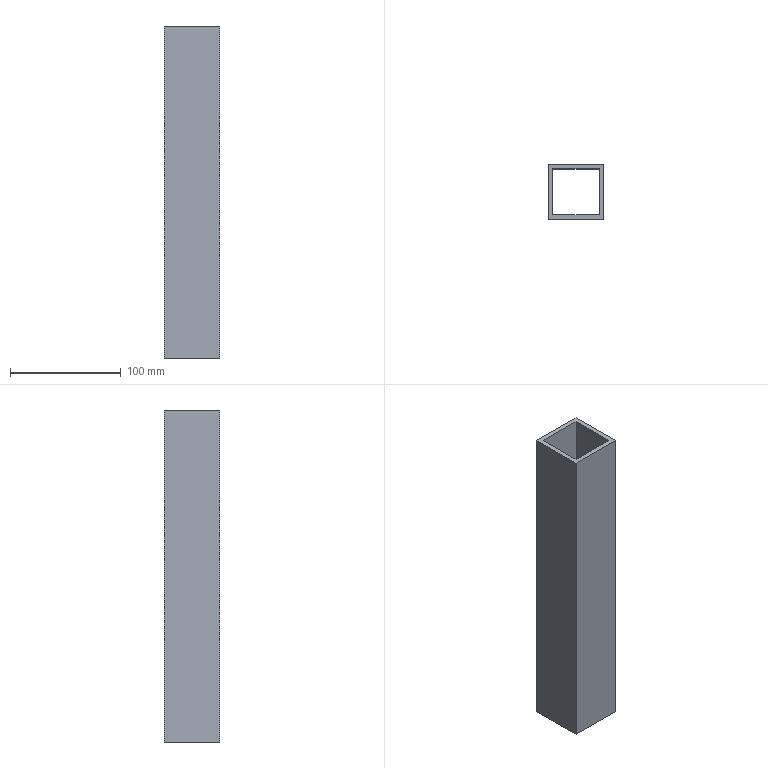Part | STEP file | PN_0083 straight stop bar | 1 solid | 10 faces | box 50 x 50 x 300 mm | volume 220800 mm3 | plane 10
STEP:
#1=CARTESIAN_POINT('',(0.,0.,0.));
#2=DIRECTION('',(0.,0.,1.));
#3=DIRECTION('',(1.,0.,0.));
#4=AXIS2_PLACEMENT_3D('',#1,#2,#3);
#5=CARTESIAN_POINT('',(-25.,25.,300.));
#6=VERTEX_POINT('',#5);
#7=CARTESIAN_POINT('',(-25.,-25.,300.));
#8=VERTEX_POINT('',#7);
#9=CARTESIAN_POINT('',(-25.,-25.,300.));
#10=DIRECTION('',(0.,-1.,0.));
#11=VECTOR('',#10,1.);
#12=LINE('',#9,#11);
#13=CARTESIAN_POINT('',(0.,0.,300.));
#14=DIRECTION('',(0.,0.,1.));
#15=DIRECTION('',(1.,0.,0.));
#16=AXIS2_PLACEMENT_3D('',#13,#14,#15);
#17=PLANE('',#16);
#18=CARTESIAN_POINT('',(-25.,-25.));
#19=DIRECTION('',(0.,-1.));
#20=VECTOR('',#19,1.);
#21=LINE('',#18,#20);
#22=(GEOMETRIC_REPRESENTATION_CONTEXT(2)PARAMETRIC_REPRESENTATION_CONTEXT()REPRESENTATION_CONTEXT('',''));
#23=DEFINITIONAL_REPRESENTATION('',(#21),#22);
#24=PCURVE('',#17,#23);
#25=CARTESIAN_POINT('',(-25.,-25.,300.));
#26=DIRECTION('',(1.,0.,0.));
#27=DIRECTION('',(0.,0.,-1.));
#28=AXIS2_PLACEMENT_3D('',#25,#26,#27);
#29=PLANE('',#28);
#30=CARTESIAN_POINT('',(0.,0.));
#31=DIRECTION('',(0.,-1.));
#32=VECTOR('',#31,1.);
#33=LINE('',#30,#32);
#34=(GEOMETRIC_REPRESENTATION_CONTEXT(2)PARAMETRIC_REPRESENTATION_CONTEXT()REPRESENTATION_CONTEXT('',''));
#35=DEFINITIONAL_REPRESENTATION('',(#33),#34);
#36=PCURVE('',#29,#35);
#37=SURFACE_CURVE('',#12,(#24,#36),.PCURVE_S1.);
#38=EDGE_CURVE('',#6,#8,#37,.T.);
#39=ORIENTED_EDGE('',*,*,#38,.T.);
#40=CARTESIAN_POINT('',(25.,-25.,300.));
#41=VERTEX_POINT('',#40);
#42=CARTESIAN_POINT('',(25.,-25.,300.));
#43=DIRECTION('',(1.,0.,0.));
#44=VECTOR('',#43,1.);
#45=LINE('',#42,#44);
#46=CARTESIAN_POINT('',(25.,-25.));
#47=DIRECTION('',(1.,0.));
#48=VECTOR('',#47,1.);
#49=LINE('',#46,#48);
#50=(GEOMETRIC_REPRESENTATION_CONTEXT(2)PARAMETRIC_REPRESENTATION_CONTEXT()REPRESENTATION_CONTEXT('',''));
#51=DEFINITIONAL_REPRESENTATION('',(#49),#50);
#52=PCURVE('',#17,#51);
#53=CARTESIAN_POINT('',(25.,-25.,300.));
#54=DIRECTION('',(0.,1.,0.));
#55=DIRECTION('',(-1.,0.,0.));
#56=AXIS2_PLACEMENT_3D('',#53,#54,#55);
#57=PLANE('',#56);
#58=CARTESIAN_POINT('',(0.,0.));
#59=DIRECTION('',(-1.,0.));
#60=VECTOR('',#59,1.);
#61=LINE('',#58,#60);
#62=(GEOMETRIC_REPRESENTATION_CONTEXT(2)PARAMETRIC_REPRESENTATION_CONTEXT()REPRESENTATION_CONTEXT('',''));
#63=DEFINITIONAL_REPRESENTATION('',(#61),#62);
#64=PCURVE('',#57,#63);
#65=SURFACE_CURVE('',#45,(#52,#64),.PCURVE_S1.);
#66=EDGE_CURVE('',#8,#41,#65,.T.);
#67=ORIENTED_EDGE('',*,*,#66,.T.);
#68=CARTESIAN_POINT('',(25.,25.,300.));
#69=VERTEX_POINT('',#68);
#70=CARTESIAN_POINT('',(25.,-25.,300.));
#71=DIRECTION('',(0.,1.,0.));
#72=VECTOR('',#71,1.);
#73=LINE('',#70,#72);
#74=CARTESIAN_POINT('',(25.,-25.));
#75=DIRECTION('',(0.,1.));
#76=VECTOR('',#75,1.);
#77=LINE('',#74,#76);
#78=(GEOMETRIC_REPRESENTATION_CONTEXT(2)PARAMETRIC_REPRESENTATION_CONTEXT()REPRESENTATION_CONTEXT('',''));
#79=DEFINITIONAL_REPRESENTATION('',(#77),#78);
#80=PCURVE('',#17,#79);
#81=CARTESIAN_POINT('',(25.,-25.,300.));
#82=DIRECTION('',(-1.,0.,0.));
#83=DIRECTION('',(0.,0.,1.));
#84=AXIS2_PLACEMENT_3D('',#81,#82,#83);
#85=PLANE('',#84);
#86=CARTESIAN_POINT('',(0.,0.));
#87=DIRECTION('',(0.,1.));
#88=VECTOR('',#87,1.);
#89=LINE('',#86,#88);
#90=(GEOMETRIC_REPRESENTATION_CONTEXT(2)PARAMETRIC_REPRESENTATION_CONTEXT()REPRESENTATION_CONTEXT('',''));
#91=DEFINITIONAL_REPRESENTATION('',(#89),#90);
#92=PCURVE('',#85,#91);
#93=SURFACE_CURVE('',#73,(#80,#92),.PCURVE_S1.);
#94=EDGE_CURVE('',#41,#69,#93,.T.);
#95=ORIENTED_EDGE('',*,*,#94,.T.);
#96=CARTESIAN_POINT('',(25.,25.,300.));
#97=DIRECTION('',(-1.,0.,0.));
#98=VECTOR('',#97,1.);
#99=LINE('',#96,#98);
#100=CARTESIAN_POINT('',(25.,25.));
#101=DIRECTION('',(-1.,0.));
#102=VECTOR('',#101,1.);
#103=LINE('',#100,#102);
#104=(GEOMETRIC_REPRESENTATION_CONTEXT(2)PARAMETRIC_REPRESENTATION_CONTEXT()REPRESENTATION_CONTEXT('',''));
#105=DEFINITIONAL_REPRESENTATION('',(#103),#104);
#106=PCURVE('',#17,#105);
#107=CARTESIAN_POINT('',(25.,25.,300.));
#108=DIRECTION('',(0.,-1.,0.));
#109=DIRECTION('',(1.,0.,0.));
#110=AXIS2_PLACEMENT_3D('',#107,#108,#109);
#111=PLANE('',#110);
#112=CARTESIAN_POINT('',(0.,0.));
#113=DIRECTION('',(-1.,0.));
#114=VECTOR('',#113,1.);
#115=LINE('',#112,#114);
#116=(GEOMETRIC_REPRESENTATION_CONTEXT(2)PARAMETRIC_REPRESENTATION_CONTEXT()REPRESENTATION_CONTEXT('',''));
#117=DEFINITIONAL_REPRESENTATION('',(#115),#116);
#118=PCURVE('',#111,#117);
#119=SURFACE_CURVE('',#99,(#106,#118),.PCURVE_S1.);
#120=EDGE_CURVE('',#69,#6,#119,.T.);
#121=ORIENTED_EDGE('',*,*,#120,.T.);
#122=EDGE_LOOP('',(#39,#67,#95,#121));
#123=FACE_BOUND('',#122,.T.);
#124=CARTESIAN_POINT('',(-21.,-21.,300.));
#125=VERTEX_POINT('',#124);
#126=CARTESIAN_POINT('',(21.,-21.,300.));
#127=VERTEX_POINT('',#126);
#128=CARTESIAN_POINT('',(21.,-21.,300.));
#129=DIRECTION('',(1.,0.,0.));
#130=VECTOR('',#129,1.);
#131=LINE('',#128,#130);
#132=CARTESIAN_POINT('',(21.,-21.));
#133=DIRECTION('',(1.,0.));
#134=VECTOR('',#133,1.);
#135=LINE('',#132,#134);
#136=(GEOMETRIC_REPRESENTATION_CONTEXT(2)PARAMETRIC_REPRESENTATION_CONTEXT()REPRESENTATION_CONTEXT('',''));
#137=DEFINITIONAL_REPRESENTATION('',(#135),#136);
#138=PCURVE('',#17,#137);
#139=CARTESIAN_POINT('',(21.,-21.,300.));
#140=DIRECTION('',(0.,1.,0.));
#141=DIRECTION('',(0.,0.,1.));
#142=AXIS2_PLACEMENT_3D('',#139,#140,#141);
#143=PLANE('',#142);
#144=CARTESIAN_POINT('',(0.,0.));
#145=DIRECTION('',(0.,1.));
#146=VECTOR('',#145,1.);
#147=LINE('',#144,#146);
#148=(GEOMETRIC_REPRESENTATION_CONTEXT(2)PARAMETRIC_REPRESENTATION_CONTEXT()REPRESENTATION_CONTEXT('',''));
#149=DEFINITIONAL_REPRESENTATION('',(#147),#148);
#150=PCURVE('',#143,#149);
#151=SURFACE_CURVE('',#131,(#138,#150),.PCURVE_S1.);
#152=EDGE_CURVE('',#125,#127,#151,.T.);
#153=ORIENTED_EDGE('',*,*,#152,.F.);
#154=CARTESIAN_POINT('',(-21.,21.,300.));
#155=VERTEX_POINT('',#154);
#156=CARTESIAN_POINT('',(-21.,-21.,300.));
#157=DIRECTION('',(0.,-1.,0.));
#158=VECTOR('',#157,1.);
#159=LINE('',#156,#158);
#160=CARTESIAN_POINT('',(-21.,-21.));
#161=DIRECTION('',(0.,-1.));
#162=VECTOR('',#161,1.);
#163=LINE('',#160,#162);
#164=(GEOMETRIC_REPRESENTATION_CONTEXT(2)PARAMETRIC_REPRESENTATION_CONTEXT()REPRESENTATION_CONTEXT('',''));
#165=DEFINITIONAL_REPRESENTATION('',(#163),#164);
#166=PCURVE('',#17,#165);
#167=CARTESIAN_POINT('',(-21.,-21.,300.));
#168=DIRECTION('',(1.,0.,0.));
#169=DIRECTION('',(0.,0.,-1.));
#170=AXIS2_PLACEMENT_3D('',#167,#168,#169);
#171=PLANE('',#170);
#172=CARTESIAN_POINT('',(0.,0.));
#173=DIRECTION('',(0.,-1.));
#174=VECTOR('',#173,1.);
#175=LINE('',#172,#174);
#176=(GEOMETRIC_REPRESENTATION_CONTEXT(2)PARAMETRIC_REPRESENTATION_CONTEXT()REPRESENTATION_CONTEXT('',''));
#177=DEFINITIONAL_REPRESENTATION('',(#175),#176);
#178=PCURVE('',#171,#177);
#179=SURFACE_CURVE('',#159,(#166,#178),.PCURVE_S1.);
#180=EDGE_CURVE('',#155,#125,#179,.T.);
#181=ORIENTED_EDGE('',*,*,#180,.F.);
#182=CARTESIAN_POINT('',(21.,21.,300.));
#183=VERTEX_POINT('',#182);
#184=CARTESIAN_POINT('',(21.,21.,300.));
#185=DIRECTION('',(-1.,0.,0.));
#186=VECTOR('',#185,1.);
#187=LINE('',#184,#186);
#188=CARTESIAN_POINT('',(21.,21.));
#189=DIRECTION('',(-1.,0.));
#190=VECTOR('',#189,1.);
#191=LINE('',#188,#190);
#192=(GEOMETRIC_REPRESENTATION_CONTEXT(2)PARAMETRIC_REPRESENTATION_CONTEXT()REPRESENTATION_CONTEXT('',''));
#193=DEFINITIONAL_REPRESENTATION('',(#191),#192);
#194=PCURVE('',#17,#193);
#195=CARTESIAN_POINT('',(21.,21.,300.));
#196=DIRECTION('',(0.,-1.,0.));
#197=DIRECTION('',(0.,0.,-1.));
#198=AXIS2_PLACEMENT_3D('',#195,#196,#197);
#199=PLANE('',#198);
#200=CARTESIAN_POINT('',(0.,0.));
#201=DIRECTION('',(0.,-1.));
#202=VECTOR('',#201,1.);
#203=LINE('',#200,#202);
#204=(GEOMETRIC_REPRESENTATION_CONTEXT(2)PARAMETRIC_REPRESENTATION_CONTEXT()REPRESENTATION_CONTEXT('',''));
#205=DEFINITIONAL_REPRESENTATION('',(#203),#204);
#206=PCURVE('',#199,#205);
#207=SURFACE_CURVE('',#187,(#194,#206),.PCURVE_S1.);
#208=EDGE_CURVE('',#183,#155,#207,.T.);
#209=ORIENTED_EDGE('',*,*,#208,.F.);
#210=CARTESIAN_POINT('',(21.,-21.,300.));
#211=DIRECTION('',(0.,1.,0.));
#212=VECTOR('',#211,1.);
#213=LINE('',#210,#212);
#214=CARTESIAN_POINT('',(21.,-21.));
#215=DIRECTION('',(0.,1.));
#216=VECTOR('',#215,1.);
#217=LINE('',#214,#216);
#218=(GEOMETRIC_REPRESENTATION_CONTEXT(2)PARAMETRIC_REPRESENTATION_CONTEXT()REPRESENTATION_CONTEXT('',''));
#219=DEFINITIONAL_REPRESENTATION('',(#217),#218);
#220=PCURVE('',#17,#219);
#221=CARTESIAN_POINT('',(21.,-21.,300.));
#222=DIRECTION('',(-1.,0.,0.));
#223=DIRECTION('',(0.,0.,1.));
#224=AXIS2_PLACEMENT_3D('',#221,#222,#223);
#225=PLANE('',#224);
#226=CARTESIAN_POINT('',(0.,0.));
#227=DIRECTION('',(0.,1.));
#228=VECTOR('',#227,1.);
#229=LINE('',#226,#228);
#230=(GEOMETRIC_REPRESENTATION_CONTEXT(2)PARAMETRIC_REPRESENTATION_CONTEXT()REPRESENTATION_CONTEXT('',''));
#231=DEFINITIONAL_REPRESENTATION('',(#229),#230);
#232=PCURVE('',#225,#231);
#233=SURFACE_CURVE('',#213,(#220,#232),.PCURVE_S1.);
#234=EDGE_CURVE('',#127,#183,#233,.T.);
#235=ORIENTED_EDGE('',*,*,#234,.F.);
#236=EDGE_LOOP('',(#153,#181,#209,#235));
#237=FACE_BOUND('',#236,.T.);
#238=ADVANCED_FACE('',(#123,#237),#17,.T.);
#239=CARTESIAN_POINT('',(-25.,25.,0.));
#240=VERTEX_POINT('',#239);
#241=CARTESIAN_POINT('',(-25.,-25.,0.));
#242=VERTEX_POINT('',#241);
#243=CARTESIAN_POINT('',(-25.,-25.,0.));
#244=DIRECTION('',(0.,-1.,0.));
#245=VECTOR('',#244,1.);
#246=LINE('',#243,#245);
#247=CARTESIAN_POINT('',(0.,0.,0.));
#248=DIRECTION('',(0.,0.,1.));
#249=DIRECTION('',(1.,0.,0.));
#250=AXIS2_PLACEMENT_3D('',#247,#248,#249);
#251=PLANE('',#250);
#252=CARTESIAN_POINT('',(-25.,-25.));
#253=DIRECTION('',(0.,-1.));
#254=VECTOR('',#253,1.);
#255=LINE('',#252,#254);
#256=(GEOMETRIC_REPRESENTATION_CONTEXT(2)PARAMETRIC_REPRESENTATION_CONTEXT()REPRESENTATION_CONTEXT('',''));
#257=DEFINITIONAL_REPRESENTATION('',(#255),#256);
#258=PCURVE('',#251,#257);
#259=CARTESIAN_POINT('',(300.,0.));
#260=DIRECTION('',(0.,-1.));
#261=VECTOR('',#260,1.);
#262=LINE('',#259,#261);
#263=(GEOMETRIC_REPRESENTATION_CONTEXT(2)PARAMETRIC_REPRESENTATION_CONTEXT()REPRESENTATION_CONTEXT('',''));
#264=DEFINITIONAL_REPRESENTATION('',(#262),#263);
#265=PCURVE('',#29,#264);
#266=SURFACE_CURVE('',#246,(#258,#265),.PCURVE_S1.);
#267=EDGE_CURVE('',#240,#242,#266,.T.);
#268=ORIENTED_EDGE('',*,*,#267,.F.);
#269=CARTESIAN_POINT('',(25.,25.,0.));
#270=VERTEX_POINT('',#269);
#271=CARTESIAN_POINT('',(25.,25.,0.));
#272=DIRECTION('',(-1.,0.,0.));
#273=VECTOR('',#272,1.);
#274=LINE('',#271,#273);
#275=CARTESIAN_POINT('',(25.,25.));
#276=DIRECTION('',(-1.,0.));
#277=VECTOR('',#276,1.);
#278=LINE('',#275,#277);
#279=(GEOMETRIC_REPRESENTATION_CONTEXT(2)PARAMETRIC_REPRESENTATION_CONTEXT()REPRESENTATION_CONTEXT('',''));
#280=DEFINITIONAL_REPRESENTATION('',(#278),#279);
#281=PCURVE('',#251,#280);
#282=CARTESIAN_POINT('',(0.,-300.));
#283=DIRECTION('',(-1.,0.));
#284=VECTOR('',#283,1.);
#285=LINE('',#282,#284);
#286=(GEOMETRIC_REPRESENTATION_CONTEXT(2)PARAMETRIC_REPRESENTATION_CONTEXT()REPRESENTATION_CONTEXT('',''));
#287=DEFINITIONAL_REPRESENTATION('',(#285),#286);
#288=PCURVE('',#111,#287);
#289=SURFACE_CURVE('',#274,(#281,#288),.PCURVE_S1.);
#290=EDGE_CURVE('',#270,#240,#289,.T.);
#291=ORIENTED_EDGE('',*,*,#290,.F.);
#292=CARTESIAN_POINT('',(25.,-25.,0.));
#293=VERTEX_POINT('',#292);
#294=CARTESIAN_POINT('',(25.,-25.,0.));
#295=DIRECTION('',(0.,1.,0.));
#296=VECTOR('',#295,1.);
#297=LINE('',#294,#296);
#298=CARTESIAN_POINT('',(25.,-25.));
#299=DIRECTION('',(0.,1.));
#300=VECTOR('',#299,1.);
#301=LINE('',#298,#300);
#302=(GEOMETRIC_REPRESENTATION_CONTEXT(2)PARAMETRIC_REPRESENTATION_CONTEXT()REPRESENTATION_CONTEXT('',''));
#303=DEFINITIONAL_REPRESENTATION('',(#301),#302);
#304=PCURVE('',#251,#303);
#305=CARTESIAN_POINT('',(-300.,0.));
#306=DIRECTION('',(0.,1.));
#307=VECTOR('',#306,1.);
#308=LINE('',#305,#307);
#309=(GEOMETRIC_REPRESENTATION_CONTEXT(2)PARAMETRIC_REPRESENTATION_CONTEXT()REPRESENTATION_CONTEXT('',''));
#310=DEFINITIONAL_REPRESENTATION('',(#308),#309);
#311=PCURVE('',#85,#310);
#312=SURFACE_CURVE('',#297,(#304,#311),.PCURVE_S1.);
#313=EDGE_CURVE('',#293,#270,#312,.T.);
#314=ORIENTED_EDGE('',*,*,#313,.F.);
#315=CARTESIAN_POINT('',(25.,-25.,0.));
#316=DIRECTION('',(1.,0.,0.));
#317=VECTOR('',#316,1.);
#318=LINE('',#315,#317);
#319=CARTESIAN_POINT('',(25.,-25.));
#320=DIRECTION('',(1.,0.));
#321=VECTOR('',#320,1.);
#322=LINE('',#319,#321);
#323=(GEOMETRIC_REPRESENTATION_CONTEXT(2)PARAMETRIC_REPRESENTATION_CONTEXT()REPRESENTATION_CONTEXT('',''));
#324=DEFINITIONAL_REPRESENTATION('',(#322),#323);
#325=PCURVE('',#251,#324);
#326=CARTESIAN_POINT('',(0.,-300.));
#327=DIRECTION('',(-1.,0.));
#328=VECTOR('',#327,1.);
#329=LINE('',#326,#328);
#330=(GEOMETRIC_REPRESENTATION_CONTEXT(2)PARAMETRIC_REPRESENTATION_CONTEXT()REPRESENTATION_CONTEXT('',''));
#331=DEFINITIONAL_REPRESENTATION('',(#329),#330);
#332=PCURVE('',#57,#331);
#333=SURFACE_CURVE('',#318,(#325,#332),.PCURVE_S1.);
#334=EDGE_CURVE('',#242,#293,#333,.T.);
#335=ORIENTED_EDGE('',*,*,#334,.F.);
#336=EDGE_LOOP('',(#268,#291,#314,#335));
#337=FACE_BOUND('',#336,.T.);
#338=CARTESIAN_POINT('',(-21.,21.,0.));
#339=VERTEX_POINT('',#338);
#340=CARTESIAN_POINT('',(-21.,-21.,0.));
#341=VERTEX_POINT('',#340);
#342=CARTESIAN_POINT('',(-21.,-21.,0.));
#343=DIRECTION('',(0.,-1.,0.));
#344=VECTOR('',#343,1.);
#345=LINE('',#342,#344);
#346=CARTESIAN_POINT('',(-21.,-21.));
#347=DIRECTION('',(0.,-1.));
#348=VECTOR('',#347,1.);
#349=LINE('',#346,#348);
#350=(GEOMETRIC_REPRESENTATION_CONTEXT(2)PARAMETRIC_REPRESENTATION_CONTEXT()REPRESENTATION_CONTEXT('',''));
#351=DEFINITIONAL_REPRESENTATION('',(#349),#350);
#352=PCURVE('',#251,#351);
#353=CARTESIAN_POINT('',(300.,0.));
#354=DIRECTION('',(0.,-1.));
#355=VECTOR('',#354,1.);
#356=LINE('',#353,#355);
#357=(GEOMETRIC_REPRESENTATION_CONTEXT(2)PARAMETRIC_REPRESENTATION_CONTEXT()REPRESENTATION_CONTEXT('',''));
#358=DEFINITIONAL_REPRESENTATION('',(#356),#357);
#359=PCURVE('',#171,#358);
#360=SURFACE_CURVE('',#345,(#352,#359),.PCURVE_S1.);
#361=EDGE_CURVE('',#339,#341,#360,.T.);
#362=ORIENTED_EDGE('',*,*,#361,.T.);
#363=CARTESIAN_POINT('',(21.,-21.,0.));
#364=VERTEX_POINT('',#363);
#365=CARTESIAN_POINT('',(21.,-21.,0.));
#366=DIRECTION('',(1.,0.,0.));
#367=VECTOR('',#366,1.);
#368=LINE('',#365,#367);
#369=CARTESIAN_POINT('',(21.,-21.));
#370=DIRECTION('',(1.,0.));
#371=VECTOR('',#370,1.);
#372=LINE('',#369,#371);
#373=(GEOMETRIC_REPRESENTATION_CONTEXT(2)PARAMETRIC_REPRESENTATION_CONTEXT()REPRESENTATION_CONTEXT('',''));
#374=DEFINITIONAL_REPRESENTATION('',(#372),#373);
#375=PCURVE('',#251,#374);
#376=CARTESIAN_POINT('',(-300.,0.));
#377=DIRECTION('',(0.,1.));
#378=VECTOR('',#377,1.);
#379=LINE('',#376,#378);
#380=(GEOMETRIC_REPRESENTATION_CONTEXT(2)PARAMETRIC_REPRESENTATION_CONTEXT()REPRESENTATION_CONTEXT('',''));
#381=DEFINITIONAL_REPRESENTATION('',(#379),#380);
#382=PCURVE('',#143,#381);
#383=SURFACE_CURVE('',#368,(#375,#382),.PCURVE_S1.);
#384=EDGE_CURVE('',#341,#364,#383,.T.);
#385=ORIENTED_EDGE('',*,*,#384,.T.);
#386=CARTESIAN_POINT('',(21.,21.,0.));
#387=VERTEX_POINT('',#386);
#388=CARTESIAN_POINT('',(21.,-21.,0.));
#389=DIRECTION('',(0.,1.,0.));
#390=VECTOR('',#389,1.);
#391=LINE('',#388,#390);
#392=CARTESIAN_POINT('',(21.,-21.));
#393=DIRECTION('',(0.,1.));
#394=VECTOR('',#393,1.);
#395=LINE('',#392,#394);
#396=(GEOMETRIC_REPRESENTATION_CONTEXT(2)PARAMETRIC_REPRESENTATION_CONTEXT()REPRESENTATION_CONTEXT('',''));
#397=DEFINITIONAL_REPRESENTATION('',(#395),#396);
#398=PCURVE('',#251,#397);
#399=CARTESIAN_POINT('',(-300.,0.));
#400=DIRECTION('',(0.,1.));
#401=VECTOR('',#400,1.);
#402=LINE('',#399,#401);
#403=(GEOMETRIC_REPRESENTATION_CONTEXT(2)PARAMETRIC_REPRESENTATION_CONTEXT()REPRESENTATION_CONTEXT('',''));
#404=DEFINITIONAL_REPRESENTATION('',(#402),#403);
#405=PCURVE('',#225,#404);
#406=SURFACE_CURVE('',#391,(#398,#405),.PCURVE_S1.);
#407=EDGE_CURVE('',#364,#387,#406,.T.);
#408=ORIENTED_EDGE('',*,*,#407,.T.);
#409=CARTESIAN_POINT('',(21.,21.,0.));
#410=DIRECTION('',(-1.,0.,0.));
#411=VECTOR('',#410,1.);
#412=LINE('',#409,#411);
#413=CARTESIAN_POINT('',(21.,21.));
#414=DIRECTION('',(-1.,0.));
#415=VECTOR('',#414,1.);
#416=LINE('',#413,#415);
#417=(GEOMETRIC_REPRESENTATION_CONTEXT(2)PARAMETRIC_REPRESENTATION_CONTEXT()REPRESENTATION_CONTEXT('',''));
#418=DEFINITIONAL_REPRESENTATION('',(#416),#417);
#419=PCURVE('',#251,#418);
#420=CARTESIAN_POINT('',(300.,0.));
#421=DIRECTION('',(0.,-1.));
#422=VECTOR('',#421,1.);
#423=LINE('',#420,#422);
#424=(GEOMETRIC_REPRESENTATION_CONTEXT(2)PARAMETRIC_REPRESENTATION_CONTEXT()REPRESENTATION_CONTEXT('',''));
#425=DEFINITIONAL_REPRESENTATION('',(#423),#424);
#426=PCURVE('',#199,#425);
#427=SURFACE_CURVE('',#412,(#419,#426),.PCURVE_S1.);
#428=EDGE_CURVE('',#387,#339,#427,.T.);
#429=ORIENTED_EDGE('',*,*,#428,.T.);
#430=EDGE_LOOP('',(#362,#385,#408,#429));
#431=FACE_BOUND('',#430,.T.);
#432=ADVANCED_FACE('',(#337,#431),#251,.F.);
#433=ORIENTED_EDGE('',*,*,#267,.T.);
#434=CARTESIAN_POINT('',(-25.,-25.,300.));
#435=DIRECTION('',(0.,0.,-1.));
#436=VECTOR('',#435,1.);
#437=LINE('',#434,#436);
#438=CARTESIAN_POINT('',(0.,0.));
#439=DIRECTION('',(1.,0.));
#440=VECTOR('',#439,1.);
#441=LINE('',#438,#440);
#442=(GEOMETRIC_REPRESENTATION_CONTEXT(2)PARAMETRIC_REPRESENTATION_CONTEXT()REPRESENTATION_CONTEXT('',''));
#443=DEFINITIONAL_REPRESENTATION('',(#441),#442);
#444=PCURVE('',#29,#443);
#445=CARTESIAN_POINT('',(50.,0.));
#446=DIRECTION('',(0.,-1.));
#447=VECTOR('',#446,1.);
#448=LINE('',#445,#447);
#449=(GEOMETRIC_REPRESENTATION_CONTEXT(2)PARAMETRIC_REPRESENTATION_CONTEXT()REPRESENTATION_CONTEXT('',''));
#450=DEFINITIONAL_REPRESENTATION('',(#448),#449);
#451=PCURVE('',#57,#450);
#452=SURFACE_CURVE('',#437,(#444,#451),.PCURVE_S1.);
#453=EDGE_CURVE('',#8,#242,#452,.T.);
#454=ORIENTED_EDGE('',*,*,#453,.F.);
#455=ORIENTED_EDGE('',*,*,#38,.F.);
#456=CARTESIAN_POINT('',(-25.,25.,300.));
#457=DIRECTION('',(0.,0.,-1.));
#458=VECTOR('',#457,1.);
#459=LINE('',#456,#458);
#460=CARTESIAN_POINT('',(0.,50.));
#461=DIRECTION('',(1.,0.));
#462=VECTOR('',#461,1.);
#463=LINE('',#460,#462);
#464=(GEOMETRIC_REPRESENTATION_CONTEXT(2)PARAMETRIC_REPRESENTATION_CONTEXT()REPRESENTATION_CONTEXT('',''));
#465=DEFINITIONAL_REPRESENTATION('',(#463),#464);
#466=PCURVE('',#29,#465);
#467=CARTESIAN_POINT('',(-50.,0.));
#468=DIRECTION('',(0.,-1.));
#469=VECTOR('',#468,1.);
#470=LINE('',#467,#469);
#471=(GEOMETRIC_REPRESENTATION_CONTEXT(2)PARAMETRIC_REPRESENTATION_CONTEXT()REPRESENTATION_CONTEXT('',''));
#472=DEFINITIONAL_REPRESENTATION('',(#470),#471);
#473=PCURVE('',#111,#472);
#474=SURFACE_CURVE('',#459,(#466,#473),.PCURVE_S1.);
#475=EDGE_CURVE('',#6,#240,#474,.T.);
#476=ORIENTED_EDGE('',*,*,#475,.T.);
#477=EDGE_LOOP('',(#433,#454,#455,#476));
#478=FACE_BOUND('',#477,.T.);
#479=ADVANCED_FACE('',(#478),#29,.F.);
#480=ORIENTED_EDGE('',*,*,#334,.T.);
#481=CARTESIAN_POINT('',(25.,-25.,300.));
#482=DIRECTION('',(0.,0.,-1.));
#483=VECTOR('',#482,1.);
#484=LINE('',#481,#483);
#485=CARTESIAN_POINT('',(0.,0.));
#486=DIRECTION('',(0.,-1.));
#487=VECTOR('',#486,1.);
#488=LINE('',#485,#487);
#489=(GEOMETRIC_REPRESENTATION_CONTEXT(2)PARAMETRIC_REPRESENTATION_CONTEXT()REPRESENTATION_CONTEXT('',''));
#490=DEFINITIONAL_REPRESENTATION('',(#488),#489);
#491=PCURVE('',#57,#490);
#492=CARTESIAN_POINT('',(0.,0.));
#493=DIRECTION('',(-1.,0.));
#494=VECTOR('',#493,1.);
#495=LINE('',#492,#494);
#496=(GEOMETRIC_REPRESENTATION_CONTEXT(2)PARAMETRIC_REPRESENTATION_CONTEXT()REPRESENTATION_CONTEXT('',''));
#497=DEFINITIONAL_REPRESENTATION('',(#495),#496);
#498=PCURVE('',#85,#497);
#499=SURFACE_CURVE('',#484,(#491,#498),.PCURVE_S1.);
#500=EDGE_CURVE('',#41,#293,#499,.T.);
#501=ORIENTED_EDGE('',*,*,#500,.F.);
#502=ORIENTED_EDGE('',*,*,#66,.F.);
#503=ORIENTED_EDGE('',*,*,#453,.T.);
#504=EDGE_LOOP('',(#480,#501,#502,#503));
#505=FACE_BOUND('',#504,.T.);
#506=ADVANCED_FACE('',(#505),#57,.F.);
#507=ORIENTED_EDGE('',*,*,#313,.T.);
#508=CARTESIAN_POINT('',(25.,25.,300.));
#509=DIRECTION('',(0.,0.,-1.));
#510=VECTOR('',#509,1.);
#511=LINE('',#508,#510);
#512=CARTESIAN_POINT('',(0.,50.));
#513=DIRECTION('',(-1.,0.));
#514=VECTOR('',#513,1.);
#515=LINE('',#512,#514);
#516=(GEOMETRIC_REPRESENTATION_CONTEXT(2)PARAMETRIC_REPRESENTATION_CONTEXT()REPRESENTATION_CONTEXT('',''));
#517=DEFINITIONAL_REPRESENTATION('',(#515),#516);
#518=PCURVE('',#85,#517);
#519=CARTESIAN_POINT('',(0.,0.));
#520=DIRECTION('',(0.,-1.));
#521=VECTOR('',#520,1.);
#522=LINE('',#519,#521);
#523=(GEOMETRIC_REPRESENTATION_CONTEXT(2)PARAMETRIC_REPRESENTATION_CONTEXT()REPRESENTATION_CONTEXT('',''));
#524=DEFINITIONAL_REPRESENTATION('',(#522),#523);
#525=PCURVE('',#111,#524);
#526=SURFACE_CURVE('',#511,(#518,#525),.PCURVE_S1.);
#527=EDGE_CURVE('',#69,#270,#526,.T.);
#528=ORIENTED_EDGE('',*,*,#527,.F.);
#529=ORIENTED_EDGE('',*,*,#94,.F.);
#530=ORIENTED_EDGE('',*,*,#500,.T.);
#531=EDGE_LOOP('',(#507,#528,#529,#530));
#532=FACE_BOUND('',#531,.T.);
#533=ADVANCED_FACE('',(#532),#85,.F.);
#534=ORIENTED_EDGE('',*,*,#290,.T.);
#535=ORIENTED_EDGE('',*,*,#475,.F.);
#536=ORIENTED_EDGE('',*,*,#120,.F.);
#537=ORIENTED_EDGE('',*,*,#527,.T.);
#538=EDGE_LOOP('',(#534,#535,#536,#537));
#539=FACE_BOUND('',#538,.T.);
#540=ADVANCED_FACE('',(#539),#111,.F.);
#541=ORIENTED_EDGE('',*,*,#361,.F.);
#542=CARTESIAN_POINT('',(-21.,21.,300.));
#543=DIRECTION('',(0.,0.,-1.));
#544=VECTOR('',#543,1.);
#545=LINE('',#542,#544);
#546=CARTESIAN_POINT('',(0.,42.));
#547=DIRECTION('',(1.,0.));
#548=VECTOR('',#547,1.);
#549=LINE('',#546,#548);
#550=(GEOMETRIC_REPRESENTATION_CONTEXT(2)PARAMETRIC_REPRESENTATION_CONTEXT()REPRESENTATION_CONTEXT('',''));
#551=DEFINITIONAL_REPRESENTATION('',(#549),#550);
#552=PCURVE('',#171,#551);
#553=CARTESIAN_POINT('',(0.,-42.));
#554=DIRECTION('',(1.,0.));
#555=VECTOR('',#554,1.);
#556=LINE('',#553,#555);
#557=(GEOMETRIC_REPRESENTATION_CONTEXT(2)PARAMETRIC_REPRESENTATION_CONTEXT()REPRESENTATION_CONTEXT('',''));
#558=DEFINITIONAL_REPRESENTATION('',(#556),#557);
#559=PCURVE('',#199,#558);
#560=SURFACE_CURVE('',#545,(#552,#559),.PCURVE_S1.);
#561=EDGE_CURVE('',#155,#339,#560,.T.);
#562=ORIENTED_EDGE('',*,*,#561,.F.);
#563=ORIENTED_EDGE('',*,*,#180,.T.);
#564=CARTESIAN_POINT('',(-21.,-21.,300.));
#565=DIRECTION('',(0.,0.,-1.));
#566=VECTOR('',#565,1.);
#567=LINE('',#564,#566);
#568=CARTESIAN_POINT('',(0.,0.));
#569=DIRECTION('',(1.,0.));
#570=VECTOR('',#569,1.);
#571=LINE('',#568,#570);
#572=(GEOMETRIC_REPRESENTATION_CONTEXT(2)PARAMETRIC_REPRESENTATION_CONTEXT()REPRESENTATION_CONTEXT('',''));
#573=DEFINITIONAL_REPRESENTATION('',(#571),#572);
#574=PCURVE('',#171,#573);
#575=CARTESIAN_POINT('',(0.,-42.));
#576=DIRECTION('',(-1.,0.));
#577=VECTOR('',#576,1.);
#578=LINE('',#575,#577);
#579=(GEOMETRIC_REPRESENTATION_CONTEXT(2)PARAMETRIC_REPRESENTATION_CONTEXT()REPRESENTATION_CONTEXT('',''));
#580=DEFINITIONAL_REPRESENTATION('',(#578),#579);
#581=PCURVE('',#143,#580);
#582=SURFACE_CURVE('',#567,(#574,#581),.PCURVE_S1.);
#583=EDGE_CURVE('',#125,#341,#582,.T.);
#584=ORIENTED_EDGE('',*,*,#583,.T.);
#585=EDGE_LOOP('',(#541,#562,#563,#584));
#586=FACE_BOUND('',#585,.T.);
#587=ADVANCED_FACE('',(#586),#171,.T.);
#588=ORIENTED_EDGE('',*,*,#384,.F.);
#589=ORIENTED_EDGE('',*,*,#583,.F.);
#590=ORIENTED_EDGE('',*,*,#152,.T.);
#591=CARTESIAN_POINT('',(21.,-21.,300.));
#592=DIRECTION('',(0.,0.,-1.));
#593=VECTOR('',#592,1.);
#594=LINE('',#591,#593);
#595=CARTESIAN_POINT('',(0.,0.));
#596=DIRECTION('',(-1.,0.));
#597=VECTOR('',#596,1.);
#598=LINE('',#595,#597);
#599=(GEOMETRIC_REPRESENTATION_CONTEXT(2)PARAMETRIC_REPRESENTATION_CONTEXT()REPRESENTATION_CONTEXT('',''));
#600=DEFINITIONAL_REPRESENTATION('',(#598),#599);
#601=PCURVE('',#143,#600);
#602=CARTESIAN_POINT('',(0.,0.));
#603=DIRECTION('',(-1.,0.));
#604=VECTOR('',#603,1.);
#605=LINE('',#602,#604);
#606=(GEOMETRIC_REPRESENTATION_CONTEXT(2)PARAMETRIC_REPRESENTATION_CONTEXT()REPRESENTATION_CONTEXT('',''));
#607=DEFINITIONAL_REPRESENTATION('',(#605),#606);
#608=PCURVE('',#225,#607);
#609=SURFACE_CURVE('',#594,(#601,#608),.PCURVE_S1.);
#610=EDGE_CURVE('',#127,#364,#609,.T.);
#611=ORIENTED_EDGE('',*,*,#610,.T.);
#612=EDGE_LOOP('',(#588,#589,#590,#611));
#613=FACE_BOUND('',#612,.T.);
#614=ADVANCED_FACE('',(#613),#143,.T.);
#615=ORIENTED_EDGE('',*,*,#407,.F.);
#616=ORIENTED_EDGE('',*,*,#610,.F.);
#617=ORIENTED_EDGE('',*,*,#234,.T.);
#618=CARTESIAN_POINT('',(21.,21.,300.));
#619=DIRECTION('',(0.,0.,-1.));
#620=VECTOR('',#619,1.);
#621=LINE('',#618,#620);
#622=CARTESIAN_POINT('',(0.,42.));
#623=DIRECTION('',(-1.,0.));
#624=VECTOR('',#623,1.);
#625=LINE('',#622,#624);
#626=(GEOMETRIC_REPRESENTATION_CONTEXT(2)PARAMETRIC_REPRESENTATION_CONTEXT()REPRESENTATION_CONTEXT('',''));
#627=DEFINITIONAL_REPRESENTATION('',(#625),#626);
#628=PCURVE('',#225,#627);
#629=CARTESIAN_POINT('',(0.,0.));
#630=DIRECTION('',(1.,0.));
#631=VECTOR('',#630,1.);
#632=LINE('',#629,#631);
#633=(GEOMETRIC_REPRESENTATION_CONTEXT(2)PARAMETRIC_REPRESENTATION_CONTEXT()REPRESENTATION_CONTEXT('',''));
#634=DEFINITIONAL_REPRESENTATION('',(#632),#633);
#635=PCURVE('',#199,#634);
#636=SURFACE_CURVE('',#621,(#628,#635),.PCURVE_S1.);
#637=EDGE_CURVE('',#183,#387,#636,.T.);
#638=ORIENTED_EDGE('',*,*,#637,.T.);
#639=EDGE_LOOP('',(#615,#616,#617,#638));
#640=FACE_BOUND('',#639,.T.);
#641=ADVANCED_FACE('',(#640),#225,.T.);
#642=ORIENTED_EDGE('',*,*,#428,.F.);
#643=ORIENTED_EDGE('',*,*,#637,.F.);
#644=ORIENTED_EDGE('',*,*,#208,.T.);
#645=ORIENTED_EDGE('',*,*,#561,.T.);
#646=EDGE_LOOP('',(#642,#643,#644,#645));
#647=FACE_BOUND('',#646,.T.);
#648=ADVANCED_FACE('',(#647),#199,.T.);
#649=CLOSED_SHELL('',(#238,#432,#479,#506,#533,#540,#587,#614,#641,#648));
#650=MANIFOLD_SOLID_BREP('',#649);
#651=(LENGTH_UNIT()NAMED_UNIT(*)SI_UNIT(.MILLI.,.METRE.));
#652=UNCERTAINTY_MEASURE_WITH_UNIT(LENGTH_MEASURE(0.0000001),#651,'','');
#653=(NAMED_UNIT(*)PLANE_ANGLE_UNIT()SI_UNIT($,.RADIAN.));
#654=(NAMED_UNIT(*)SI_UNIT($,.STERADIAN.)SOLID_ANGLE_UNIT());
#655=(GEOMETRIC_REPRESENTATION_CONTEXT(3)GLOBAL_UNCERTAINTY_ASSIGNED_CONTEXT((#652))GLOBAL_UNIT_ASSIGNED_CONTEXT((#651,#653,#654))REPRESENTATION_CONTEXT('',''));
#656=ADVANCED_BREP_SHAPE_REPRESENTATION('',(#4,#650),#655);